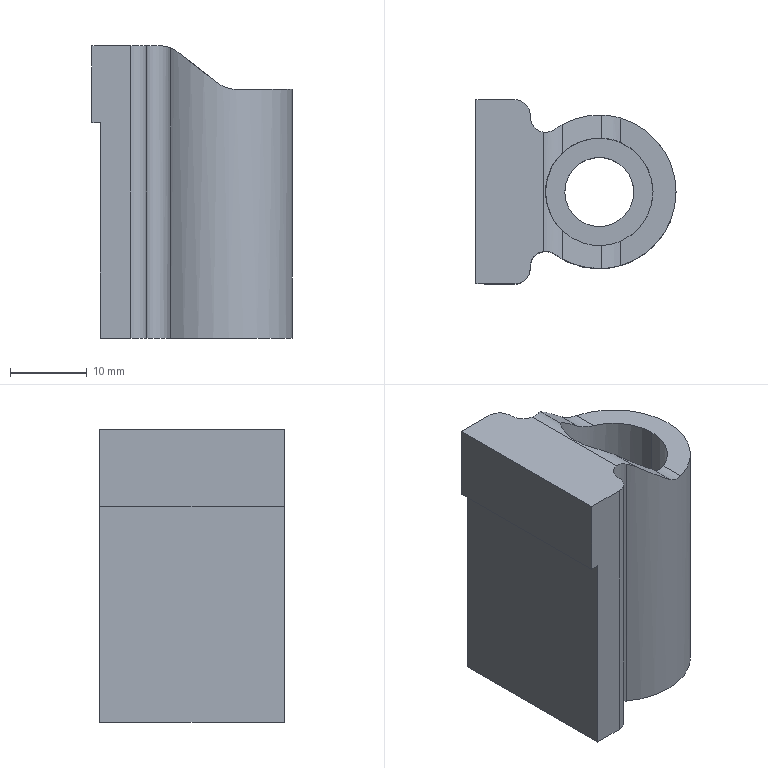Part | STEP file | 1_id810_x_t | 1 solid | 25 faces | box 26.07 x 24 x 38.1 mm | volume 13100 mm3 | plane 13 | cylinder 12 | commonest cylinder face diameters 4 x4 8 x3 9 x2 14 x2 20 x1